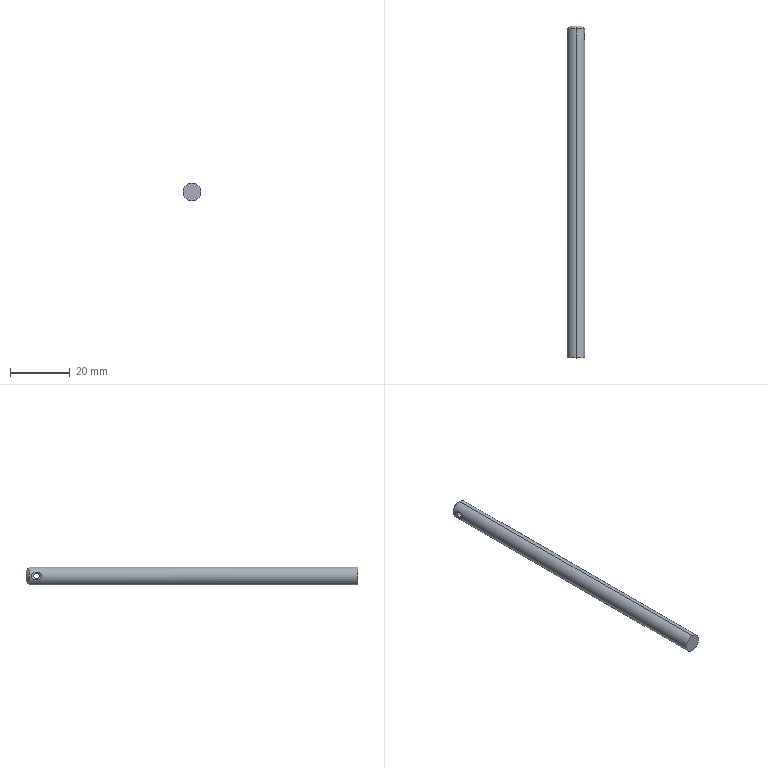Part | SolidWorks | features ICE 2, Chamfer 1, Extrusion 1, MirrorPattern 1 | 1 solid | 12 faces | box 6 x 111 x 6 mm | volume 3110 mm3 | cone 6 | cylinder 4 | plane 2 | commonest cylinder face diameters 2 x2 6 x2
STEP:
#1=CARTESIAN_POINT('',(0.,111.,2.));
#2=VERTEX_POINT('',#1);
#3=CARTESIAN_POINT('',(0.,111.,-2.));
#4=VERTEX_POINT('',#3);
#5=CARTESIAN_POINT('',(0.,111.,0.));
#6=DIRECTION('',(0.,1.,0.));
#7=DIRECTION('',(0.,0.,1.));
#8=AXIS2_PLACEMENT_3D('',#5,#6,#7);
#9=CIRCLE('',#8,2.);
#10=EDGE_CURVE('',#2,#4,#9,.T.);
#11=ORIENTED_EDGE('',*,*,#10,.F.);
#12=CARTESIAN_POINT('',(0.,110.,3.));
#13=VERTEX_POINT('',#12);
#14=CARTESIAN_POINT('',(0.,111.,2.));
#15=DIRECTION('',(0.,-0.7071,0.7071));
#16=VECTOR('',#15,1000.);
#17=LINE('',#14,#16);
#18=EDGE_CURVE('',#2,#13,#17,.T.);
#19=ORIENTED_EDGE('',*,*,#18,.T.);
#20=CARTESIAN_POINT('',(0.,110.,-3.));
#21=VERTEX_POINT('',#20);
#22=CARTESIAN_POINT('',(0.,110.,0.));
#23=DIRECTION('',(0.,-1.,0.));
#24=DIRECTION('',(0.,0.,1.));
#25=AXIS2_PLACEMENT_3D('',#22,#23,#24);
#26=CIRCLE('',#25,3.);
#27=EDGE_CURVE('',#21,#13,#26,.T.);
#28=ORIENTED_EDGE('',*,*,#27,.F.);
#29=CARTESIAN_POINT('',(0.,111.,-2.));
#30=DIRECTION('',(0.,-0.7071,-0.7071));
#31=VECTOR('',#30,1000.);
#32=LINE('',#29,#31);
#33=EDGE_CURVE('',#4,#21,#32,.T.);
#34=ORIENTED_EDGE('',*,*,#33,.F.);
#35=EDGE_LOOP('',(#11,#19,#28,#34));
#36=FACE_OUTER_BOUND('',#35,.T.);
#37=CARTESIAN_POINT('',(0.,111.,0.));
#38=DIRECTION('',(0.,-1.,0.));
#39=DIRECTION('',(0.,0.,-1.));
#40=AXIS2_PLACEMENT_3D('',#37,#38,#39);
#41=CONICAL_SURFACE('',#40,2.,0.7854);
#42=ADVANCED_FACE('',(#36),#41,.T.);
#43=CARTESIAN_POINT('',(-2.567,107.5,-1.));
#44=VERTEX_POINT('',#43);
#45=CARTESIAN_POINT('',(-2.567,107.5,1.));
#46=VERTEX_POINT('',#45);
#47=CARTESIAN_POINT('',(-2.567,107.5,0.));
#48=DIRECTION('',(1.,0.,0.));
#49=DIRECTION('',(0.,0.,1.));
#50=AXIS2_PLACEMENT_3D('',#47,#48,#49);
#51=CIRCLE('',#50,1.);
#52=EDGE_CURVE('',#44,#46,#51,.T.);
#53=ORIENTED_EDGE('',*,*,#52,.T.);
#54=CARTESIAN_POINT('',(-2.72,107.5,1.265));
#55=VERTEX_POINT('',#54);
#56=CARTESIAN_POINT('',(-3.,107.5,1.75));
#57=DIRECTION('',(-0.5,0.,0.866));
#58=VECTOR('',#57,1000.);
#59=LINE('',#56,#58);
#60=EDGE_CURVE('',#46,#55,#59,.T.);
#61=ORIENTED_EDGE('',*,*,#60,.T.);
#62=CARTESIAN_POINT('',(-2.72,107.5,-1.265));
#63=VERTEX_POINT('',#62);
#64=CARTESIAN_POINT('',(-2.72,107.5,1.265));
#65=CARTESIAN_POINT('',(-2.72,107.7,1.265));
#66=CARTESIAN_POINT('',(-2.733,107.897,1.24));
#67=CARTESIAN_POINT('',(-2.777,108.281,1.136));
#68=CARTESIAN_POINT('',(-2.809,108.463,1.059));
#69=CARTESIAN_POINT('',(-2.861,108.712,0.9041));
#70=CARTESIAN_POINT('',(-2.879,108.792,0.8448));
#71=CARTESIAN_POINT('',(-2.915,108.938,0.713));
#72=CARTESIAN_POINT('',(-2.932,109.004,0.6404));
#73=CARTESIAN_POINT('',(-2.963,109.12,0.4774));
#74=CARTESIAN_POINT('',(-2.976,109.166,0.39));
#75=CARTESIAN_POINT('',(-2.995,109.232,0.2007));
#76=CARTESIAN_POINT('',(-3.,109.25,0.1015));
#77=CARTESIAN_POINT('',(-3.,109.25,-0.09834));
#78=CARTESIAN_POINT('',(-2.995,109.233,-0.1991));
#79=CARTESIAN_POINT('',(-2.976,109.167,-0.388));
#80=CARTESIAN_POINT('',(-2.963,109.12,-0.4769));
#81=CARTESIAN_POINT('',(-2.932,109.006,-0.6382));
#82=CARTESIAN_POINT('',(-2.915,108.939,-0.7124));
#83=CARTESIAN_POINT('',(-2.88,108.793,-0.8441));
#84=CARTESIAN_POINT('',(-2.862,108.715,-0.9024));
#85=CARTESIAN_POINT('',(-2.809,108.464,-1.059));
#86=CARTESIAN_POINT('',(-2.777,108.281,-1.136));
#87=CARTESIAN_POINT('',(-2.733,107.899,-1.239));
#88=CARTESIAN_POINT('',(-2.72,107.699,-1.265));
#89=CARTESIAN_POINT('',(-2.72,107.5,-1.265));
#90=B_SPLINE_CURVE_WITH_KNOTS('',3,(#64,#65,#66,#67,#68,#69,#70,#71,#72,#73,#74,#75,#76,#77,#78,#79,#80,#81,#82,#83,#84,#85,#86,#87,#88,#89),.UNSPECIFIED.,.F.,.F.,(4,2,2,2,2,2,2,2,2,2,2,2,4),(0.003652,0.004246,0.00484,0.005137,0.005434,0.005731,0.006028,0.006325,0.006622,0.006919,0.007216,0.00781,0.008404),.UNSPECIFIED.);
#91=EDGE_CURVE('',#55,#63,#90,.T.);
#92=ORIENTED_EDGE('',*,*,#91,.T.);
#93=CARTESIAN_POINT('',(-3.,107.5,-1.75));
#94=DIRECTION('',(-0.5,0.,-0.866));
#95=VECTOR('',#94,1000.);
#96=LINE('',#93,#95);
#97=EDGE_CURVE('',#44,#63,#96,.T.);
#98=ORIENTED_EDGE('',*,*,#97,.F.);
#99=EDGE_LOOP('',(#53,#61,#92,#98));
#100=FACE_OUTER_BOUND('',#99,.T.);
#101=CARTESIAN_POINT('',(-3.,107.5,0.));
#102=DIRECTION('',(-1.,0.,0.));
#103=DIRECTION('',(0.,0.,-1.));
#104=AXIS2_PLACEMENT_3D('',#101,#102,#103);
#105=CONICAL_SURFACE('',#104,1.75,1.047);
#106=ADVANCED_FACE('',(#100),#105,.F.);
#107=CARTESIAN_POINT('',(2.567,107.5,1.));
#108=VERTEX_POINT('',#107);
#109=CARTESIAN_POINT('',(2.567,107.5,-1.));
#110=VERTEX_POINT('',#109);
#111=CARTESIAN_POINT('',(2.567,107.5,0.));
#112=DIRECTION('',(1.,0.,0.));
#113=DIRECTION('',(0.,0.,-1.));
#114=AXIS2_PLACEMENT_3D('',#111,#112,#113);
#115=CIRCLE('',#114,1.);
#116=EDGE_CURVE('',#108,#110,#115,.T.);
#117=ORIENTED_EDGE('',*,*,#116,.F.);
#118=CARTESIAN_POINT('',(2.72,107.5,1.265));
#119=VERTEX_POINT('',#118);
#120=CARTESIAN_POINT('',(3.,107.5,1.75));
#121=DIRECTION('',(0.5,0.,0.866));
#122=VECTOR('',#121,1000.);
#123=LINE('',#120,#122);
#124=EDGE_CURVE('',#108,#119,#123,.T.);
#125=ORIENTED_EDGE('',*,*,#124,.T.);
#126=CARTESIAN_POINT('',(2.72,107.5,-1.265));
#127=VERTEX_POINT('',#126);
#128=CARTESIAN_POINT('',(2.72,107.5,-1.265));
#129=CARTESIAN_POINT('',(2.72,107.301,-1.265));
#130=CARTESIAN_POINT('',(2.733,107.1,-1.239));
#131=CARTESIAN_POINT('',(2.777,106.72,-1.136));
#132=CARTESIAN_POINT('',(2.809,106.534,-1.058));
#133=CARTESIAN_POINT('',(2.862,106.285,-0.9018));
#134=CARTESIAN_POINT('',(2.88,106.206,-0.8437));
#135=CARTESIAN_POINT('',(2.915,106.062,-0.7128));
#136=CARTESIAN_POINT('',(2.932,105.994,-0.6389));
#137=CARTESIAN_POINT('',(2.963,105.881,-0.4775));
#138=CARTESIAN_POINT('',(2.976,105.833,-0.3889));
#139=CARTESIAN_POINT('',(2.995,105.768,-0.2005));
#140=CARTESIAN_POINT('',(3.,105.75,-0.103));
#141=CARTESIAN_POINT('',(3.,105.75,0.2009));
#142=CARTESIAN_POINT('',(2.979,105.822,0.3946));
#143=CARTESIAN_POINT('',(2.932,105.994,0.639));
#144=CARTESIAN_POINT('',(2.915,106.06,0.7115));
#145=CARTESIAN_POINT('',(2.88,106.206,0.8433));
#146=CARTESIAN_POINT('',(2.861,106.286,0.9027));
#147=CARTESIAN_POINT('',(2.809,106.536,1.058));
#148=CARTESIAN_POINT('',(2.777,106.719,1.135));
#149=CARTESIAN_POINT('',(2.733,107.102,1.239));
#150=CARTESIAN_POINT('',(2.72,107.3,1.265));
#151=CARTESIAN_POINT('',(2.72,107.5,1.265));
#152=B_SPLINE_CURVE_WITH_KNOTS('',3,(#128,#129,#130,#131,#132,#133,#134,#135,#136,#137,#138,#139,#140,#141,#142,#143,#144,#145,#146,#147,#148,#149,#150,#151),.UNSPECIFIED.,.F.,.F.,(4,2,2,2,2,2,2,2,2,2,2,4),(0.008404,0.008997,0.009591,0.009888,0.01018,0.01048,0.01078,0.01137,0.01167,0.01197,0.01256,0.01315),.UNSPECIFIED.);
#153=EDGE_CURVE('',#127,#119,#152,.T.);
#154=ORIENTED_EDGE('',*,*,#153,.F.);
#155=CARTESIAN_POINT('',(3.,107.5,-1.75));
#156=DIRECTION('',(0.5,0.,-0.866));
#157=VECTOR('',#156,1000.);
#158=LINE('',#155,#157);
#159=EDGE_CURVE('',#110,#127,#158,.T.);
#160=ORIENTED_EDGE('',*,*,#159,.F.);
#161=EDGE_LOOP('',(#117,#125,#154,#160));
#162=FACE_OUTER_BOUND('',#161,.T.);
#163=CARTESIAN_POINT('',(3.,107.5,0.));
#164=DIRECTION('',(1.,0.,0.));
#165=DIRECTION('',(0.,0.,-1.));
#166=AXIS2_PLACEMENT_3D('',#163,#164,#165);
#167=CONICAL_SURFACE('',#166,1.75,1.047);
#168=ADVANCED_FACE('',(#162),#167,.F.);
#169=CARTESIAN_POINT('',(-2.567,107.5,0.));
#170=DIRECTION('',(1.,0.,0.));
#171=DIRECTION('',(0.,0.,1.));
#172=AXIS2_PLACEMENT_3D('',#169,#170,#171);
#173=CIRCLE('',#172,1.);
#174=EDGE_CURVE('',#46,#44,#173,.T.);
#175=ORIENTED_EDGE('',*,*,#174,.F.);
#176=CARTESIAN_POINT('',(-3.,107.5,1.));
#177=DIRECTION('',(1.,0.,0.));
#178=VECTOR('',#177,1000.);
#179=LINE('',#176,#178);
#180=EDGE_CURVE('',#46,#108,#179,.T.);
#181=ORIENTED_EDGE('',*,*,#180,.T.);
#182=ORIENTED_EDGE('',*,*,#116,.T.);
#183=CARTESIAN_POINT('',(-3.,107.5,-1.));
#184=DIRECTION('',(1.,0.,0.));
#185=VECTOR('',#184,1000.);
#186=LINE('',#183,#185);
#187=EDGE_CURVE('',#44,#110,#186,.T.);
#188=ORIENTED_EDGE('',*,*,#187,.F.);
#189=EDGE_LOOP('',(#175,#181,#182,#188));
#190=FACE_OUTER_BOUND('',#189,.T.);
#191=CARTESIAN_POINT('',(-3.,107.5,0.));
#192=DIRECTION('',(1.,0.,0.));
#193=DIRECTION('',(0.,0.,-1.));
#194=AXIS2_PLACEMENT_3D('',#191,#192,#193);
#195=CYLINDRICAL_SURFACE('',#194,1.);
#196=ADVANCED_FACE('',(#190),#195,.F.);
#197=ORIENTED_EDGE('',*,*,#153,.T.);
#198=CARTESIAN_POINT('',(2.72,107.5,1.265));
#199=CARTESIAN_POINT('',(2.72,107.7,1.265));
#200=CARTESIAN_POINT('',(2.733,107.897,1.24));
#201=CARTESIAN_POINT('',(2.777,108.281,1.136));
#202=CARTESIAN_POINT('',(2.809,108.463,1.059));
#203=CARTESIAN_POINT('',(2.861,108.712,0.9041));
#204=CARTESIAN_POINT('',(2.879,108.792,0.8448));
#205=CARTESIAN_POINT('',(2.915,108.938,0.713));
#206=CARTESIAN_POINT('',(2.932,109.004,0.6404));
#207=CARTESIAN_POINT('',(2.963,109.12,0.4774));
#208=CARTESIAN_POINT('',(2.976,109.166,0.39));
#209=CARTESIAN_POINT('',(2.995,109.232,0.2007));
#210=CARTESIAN_POINT('',(3.,109.25,0.1015));
#211=CARTESIAN_POINT('',(3.,109.25,-0.09834));
#212=CARTESIAN_POINT('',(2.995,109.233,-0.1991));
#213=CARTESIAN_POINT('',(2.976,109.167,-0.388));
#214=CARTESIAN_POINT('',(2.963,109.12,-0.4769));
#215=CARTESIAN_POINT('',(2.932,109.006,-0.6382));
#216=CARTESIAN_POINT('',(2.915,108.939,-0.7124));
#217=CARTESIAN_POINT('',(2.88,108.793,-0.8441));
#218=CARTESIAN_POINT('',(2.862,108.715,-0.9024));
#219=CARTESIAN_POINT('',(2.809,108.464,-1.059));
#220=CARTESIAN_POINT('',(2.777,108.281,-1.136));
#221=CARTESIAN_POINT('',(2.733,107.899,-1.239));
#222=CARTESIAN_POINT('',(2.72,107.699,-1.265));
#223=CARTESIAN_POINT('',(2.72,107.5,-1.265));
#224=B_SPLINE_CURVE_WITH_KNOTS('',3,(#198,#199,#200,#201,#202,#203,#204,#205,#206,#207,#208,#209,#210,#211,#212,#213,#214,#215,#216,#217,#218,#219,#220,#221,#222,#223),.UNSPECIFIED.,.F.,.F.,(4,2,2,2,2,2,2,2,2,2,2,2,4),(0.003652,0.004246,0.00484,0.005137,0.005434,0.005731,0.006028,0.006325,0.006622,0.006919,0.007216,0.00781,0.008404),.UNSPECIFIED.);
#225=EDGE_CURVE('',#119,#127,#224,.T.);
#226=ORIENTED_EDGE('',*,*,#225,.T.);
#227=EDGE_LOOP('',(#197,#226));
#228=FACE_BOUND('',#227,.T.);
#229=ORIENTED_EDGE('',*,*,#27,.T.);
#230=CARTESIAN_POINT('',(0.,0.,3.));
#231=VERTEX_POINT('',#230);
#232=CARTESIAN_POINT('',(0.,111.,3.));
#233=DIRECTION('',(0.,-1.,0.));
#234=VECTOR('',#233,1000.);
#235=LINE('',#232,#234);
#236=EDGE_CURVE('',#13,#231,#235,.T.);
#237=ORIENTED_EDGE('',*,*,#236,.T.);
#238=CARTESIAN_POINT('',(0.,0.,-3.));
#239=VERTEX_POINT('',#238);
#240=CARTESIAN_POINT('',(0.,0.,0.));
#241=DIRECTION('',(0.,1.,0.));
#242=DIRECTION('',(0.,0.,1.));
#243=AXIS2_PLACEMENT_3D('',#240,#241,#242);
#244=CIRCLE('',#243,3.);
#245=EDGE_CURVE('',#231,#239,#244,.T.);
#246=ORIENTED_EDGE('',*,*,#245,.T.);
#247=CARTESIAN_POINT('',(0.,111.,-3.));
#248=DIRECTION('',(0.,-1.,0.));
#249=VECTOR('',#248,1000.);
#250=LINE('',#247,#249);
#251=EDGE_CURVE('',#21,#239,#250,.T.);
#252=ORIENTED_EDGE('',*,*,#251,.F.);
#253=EDGE_LOOP('',(#229,#237,#246,#252));
#254=FACE_OUTER_BOUND('',#253,.T.);
#255=CARTESIAN_POINT('',(0.,111.,0.));
#256=DIRECTION('',(0.,-1.,0.));
#257=DIRECTION('',(0.,0.,-1.));
#258=AXIS2_PLACEMENT_3D('',#255,#256,#257);
#259=CYLINDRICAL_SURFACE('',#258,3.);
#260=ADVANCED_FACE('',(#228,#254),#259,.T.);
#261=ORIENTED_EDGE('',*,*,#236,.F.);
#262=CARTESIAN_POINT('',(0.,110.,0.));
#263=DIRECTION('',(0.,-1.,0.));
#264=DIRECTION('',(0.,0.,1.));
#265=AXIS2_PLACEMENT_3D('',#262,#263,#264);
#266=CIRCLE('',#265,3.);
#267=EDGE_CURVE('',#13,#21,#266,.T.);
#268=ORIENTED_EDGE('',*,*,#267,.T.);
#269=ORIENTED_EDGE('',*,*,#251,.T.);
#270=CARTESIAN_POINT('',(0.,0.,0.));
#271=DIRECTION('',(0.,1.,0.));
#272=DIRECTION('',(0.,0.,1.));
#273=AXIS2_PLACEMENT_3D('',#270,#271,#272);
#274=CIRCLE('',#273,3.);
#275=EDGE_CURVE('',#239,#231,#274,.T.);
#276=ORIENTED_EDGE('',*,*,#275,.T.);
#277=EDGE_LOOP('',(#261,#268,#269,#276));
#278=FACE_OUTER_BOUND('',#277,.T.);
#279=CARTESIAN_POINT('',(-2.72,107.5,-1.265));
#280=CARTESIAN_POINT('',(-2.72,107.301,-1.265));
#281=CARTESIAN_POINT('',(-2.733,107.1,-1.239));
#282=CARTESIAN_POINT('',(-2.777,106.72,-1.136));
#283=CARTESIAN_POINT('',(-2.809,106.534,-1.058));
#284=CARTESIAN_POINT('',(-2.862,106.285,-0.9018));
#285=CARTESIAN_POINT('',(-2.88,106.206,-0.8437));
#286=CARTESIAN_POINT('',(-2.915,106.062,-0.7128));
#287=CARTESIAN_POINT('',(-2.932,105.994,-0.6389));
#288=CARTESIAN_POINT('',(-2.963,105.881,-0.4775));
#289=CARTESIAN_POINT('',(-2.976,105.833,-0.3889));
#290=CARTESIAN_POINT('',(-2.995,105.768,-0.2005));
#291=CARTESIAN_POINT('',(-3.,105.75,-0.103));
#292=CARTESIAN_POINT('',(-3.,105.75,0.2009));
#293=CARTESIAN_POINT('',(-2.979,105.822,0.3946));
#294=CARTESIAN_POINT('',(-2.932,105.994,0.639));
#295=CARTESIAN_POINT('',(-2.915,106.06,0.7115));
#296=CARTESIAN_POINT('',(-2.88,106.206,0.8433));
#297=CARTESIAN_POINT('',(-2.861,106.286,0.9027));
#298=CARTESIAN_POINT('',(-2.809,106.536,1.058));
#299=CARTESIAN_POINT('',(-2.777,106.719,1.135));
#300=CARTESIAN_POINT('',(-2.733,107.102,1.239));
#301=CARTESIAN_POINT('',(-2.72,107.3,1.265));
#302=CARTESIAN_POINT('',(-2.72,107.5,1.265));
#303=B_SPLINE_CURVE_WITH_KNOTS('',3,(#279,#280,#281,#282,#283,#284,#285,#286,#287,#288,#289,#290,#291,#292,#293,#294,#295,#296,#297,#298,#299,#300,#301,#302),.UNSPECIFIED.,.F.,.F.,(4,2,2,2,2,2,2,2,2,2,2,4),(0.008404,0.008997,0.009591,0.009888,0.01018,0.01048,0.01078,0.01137,0.01167,0.01197,0.01256,0.01315),.UNSPECIFIED.);
#304=EDGE_CURVE('',#63,#55,#303,.T.);
#305=ORIENTED_EDGE('',*,*,#304,.F.);
#306=ORIENTED_EDGE('',*,*,#91,.F.);
#307=EDGE_LOOP('',(#305,#306));
#308=FACE_BOUND('',#307,.T.);
#309=CARTESIAN_POINT('',(0.,111.,0.));
#310=DIRECTION('',(0.,-1.,0.));
#311=DIRECTION('',(0.,0.,-1.));
#312=AXIS2_PLACEMENT_3D('',#309,#310,#311);
#313=CYLINDRICAL_SURFACE('',#312,3.);
#314=ADVANCED_FACE('',(#278,#308),#313,.T.);
#315=ORIENTED_EDGE('',*,*,#180,.F.);
#316=ORIENTED_EDGE('',*,*,#52,.F.);
#317=ORIENTED_EDGE('',*,*,#187,.T.);
#318=CARTESIAN_POINT('',(2.567,107.5,0.));
#319=DIRECTION('',(1.,0.,0.));
#320=DIRECTION('',(0.,0.,-1.));
#321=AXIS2_PLACEMENT_3D('',#318,#319,#320);
#322=CIRCLE('',#321,1.);
#323=EDGE_CURVE('',#110,#108,#322,.T.);
#324=ORIENTED_EDGE('',*,*,#323,.T.);
#325=EDGE_LOOP('',(#315,#316,#317,#324));
#326=FACE_OUTER_BOUND('',#325,.T.);
#327=CARTESIAN_POINT('',(-3.,107.5,0.));
#328=DIRECTION('',(1.,0.,0.));
#329=DIRECTION('',(0.,0.,-1.));
#330=AXIS2_PLACEMENT_3D('',#327,#328,#329);
#331=CYLINDRICAL_SURFACE('',#330,1.);
#332=ADVANCED_FACE('',(#326),#331,.F.);
#333=CARTESIAN_POINT('',(0.,111.,0.));
#334=DIRECTION('',(0.,1.,0.));
#335=DIRECTION('',(0.,0.,1.));
#336=AXIS2_PLACEMENT_3D('',#333,#334,#335);
#337=CIRCLE('',#336,2.);
#338=EDGE_CURVE('',#4,#2,#337,.T.);
#339=ORIENTED_EDGE('',*,*,#338,.T.);
#340=ORIENTED_EDGE('',*,*,#10,.T.);
#341=EDGE_LOOP('',(#339,#340));
#342=FACE_OUTER_BOUND('',#341,.T.);
#343=CARTESIAN_POINT('',(0.,111.,0.));
#344=DIRECTION('',(0.,1.,0.));
#345=DIRECTION('',(0.,0.,1.));
#346=AXIS2_PLACEMENT_3D('',#343,#344,#345);
#347=PLANE('',#346);
#348=ADVANCED_FACE('',(#342),#347,.T.);
#349=ORIENTED_EDGE('',*,*,#275,.F.);
#350=ORIENTED_EDGE('',*,*,#245,.F.);
#351=EDGE_LOOP('',(#349,#350));
#352=FACE_OUTER_BOUND('',#351,.T.);
#353=CARTESIAN_POINT('',(0.,0.,0.));
#354=DIRECTION('',(0.,1.,0.));
#355=DIRECTION('',(0.,0.,1.));
#356=AXIS2_PLACEMENT_3D('',#353,#354,#355);
#357=PLANE('',#356);
#358=ADVANCED_FACE('',(#352),#357,.F.);
#359=ORIENTED_EDGE('',*,*,#124,.F.);
#360=ORIENTED_EDGE('',*,*,#323,.F.);
#361=ORIENTED_EDGE('',*,*,#159,.T.);
#362=ORIENTED_EDGE('',*,*,#225,.F.);
#363=EDGE_LOOP('',(#359,#360,#361,#362));
#364=FACE_OUTER_BOUND('',#363,.T.);
#365=CARTESIAN_POINT('',(3.,107.5,0.));
#366=DIRECTION('',(1.,0.,0.));
#367=DIRECTION('',(0.,0.,-1.));
#368=AXIS2_PLACEMENT_3D('',#365,#366,#367);
#369=CONICAL_SURFACE('',#368,1.75,1.047);
#370=ADVANCED_FACE('',(#364),#369,.F.);
#371=ORIENTED_EDGE('',*,*,#60,.F.);
#372=ORIENTED_EDGE('',*,*,#174,.T.);
#373=ORIENTED_EDGE('',*,*,#97,.T.);
#374=ORIENTED_EDGE('',*,*,#304,.T.);
#375=EDGE_LOOP('',(#371,#372,#373,#374));
#376=FACE_OUTER_BOUND('',#375,.T.);
#377=CARTESIAN_POINT('',(-3.,107.5,0.));
#378=DIRECTION('',(-1.,0.,0.));
#379=DIRECTION('',(0.,0.,-1.));
#380=AXIS2_PLACEMENT_3D('',#377,#378,#379);
#381=CONICAL_SURFACE('',#380,1.75,1.047);
#382=ADVANCED_FACE('',(#376),#381,.F.);
#383=ORIENTED_EDGE('',*,*,#18,.F.);
#384=ORIENTED_EDGE('',*,*,#338,.F.);
#385=ORIENTED_EDGE('',*,*,#33,.T.);
#386=ORIENTED_EDGE('',*,*,#267,.F.);
#387=EDGE_LOOP('',(#383,#384,#385,#386));
#388=FACE_OUTER_BOUND('',#387,.T.);
#389=CARTESIAN_POINT('',(0.,111.,0.));
#390=DIRECTION('',(0.,-1.,0.));
#391=DIRECTION('',(0.,0.,-1.));
#392=AXIS2_PLACEMENT_3D('',#389,#390,#391);
#393=CONICAL_SURFACE('',#392,2.,0.7854);
#394=ADVANCED_FACE('',(#388),#393,.T.);
#395=CLOSED_SHELL('',(#42,#106,#168,#196,#260,#314,#332,#348,#358,#370,#382,#394));
#396=MANIFOLD_SOLID_BREP('',#395);
#397=CARTESIAN_POINT('',(0.,0.,0.));
#398=DIRECTION('',(0.,0.,1.));
#399=DIRECTION('',(1.,0.,0.));
#400=AXIS2_PLACEMENT_3D('',#397,#398,#399);
#401=(LENGTH_UNIT()NAMED_UNIT(*)SI_UNIT(.MILLI.,.METRE.));
#402=UNCERTAINTY_MEASURE_WITH_UNIT(LENGTH_MEASURE(0.00001),#401,'','');
#403=(NAMED_UNIT(*)PLANE_ANGLE_UNIT()SI_UNIT($,.RADIAN.));
#404=(NAMED_UNIT(*)SI_UNIT($,.STERADIAN.)SOLID_ANGLE_UNIT());
#405=(GEOMETRIC_REPRESENTATION_CONTEXT(3)GLOBAL_UNCERTAINTY_ASSIGNED_CONTEXT((#402))GLOBAL_UNIT_ASSIGNED_CONTEXT((#401,#403,#404))REPRESENTATION_CONTEXT('',''));
#406=ADVANCED_BREP_SHAPE_REPRESENTATION('',(#396,#400),#405);